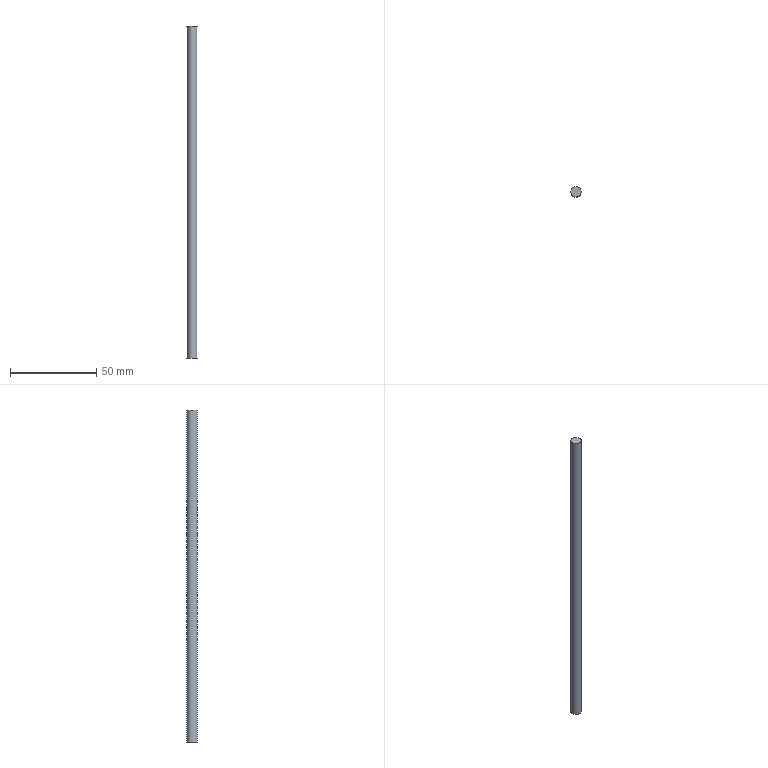Part | NX | features solid 2 | 1 solid | 3 faces | box 6 x 6 x 192 mm | volume 5429 mm3 | plane 2 | cylinder 1 | commonest cylinder face diameters 6 x1
STEP:
#1=CARTESIAN_POINT('',(276.,-28.,-282.));
#2=VERTEX_POINT('',#1);
#3=CARTESIAN_POINT('',(276.,-31.,-282.));
#4=DIRECTION('',(0.,0.,1.));
#5=DIRECTION('',(0.,1.,0.));
#6=AXIS2_PLACEMENT_3D('',#3,#4,#5);
#7=CIRCLE('',#6,3.);
#8=EDGE_CURVE('',#2,#2,#7,.T.);
#9=ORIENTED_EDGE('',*,*,#8,.T.);
#10=EDGE_LOOP('',(#9));
#11=FACE_BOUND('',#10,.T.);
#12=CARTESIAN_POINT('',(276.,-28.,-90.));
#13=VERTEX_POINT('',#12);
#14=CARTESIAN_POINT('',(276.,-31.,-90.));
#15=DIRECTION('',(0.,0.,1.));
#16=DIRECTION('',(0.,1.,0.));
#17=AXIS2_PLACEMENT_3D('',#14,#15,#16);
#18=CIRCLE('',#17,3.);
#19=EDGE_CURVE('',#13,#13,#18,.T.);
#20=ORIENTED_EDGE('',*,*,#19,.F.);
#21=EDGE_LOOP('',(#20));
#22=FACE_BOUND('',#21,.T.);
#23=CARTESIAN_POINT('',(276.,-31.,-282.));
#24=DIRECTION('',(0.,0.,1.));
#25=DIRECTION('',(0.,1.,0.));
#26=AXIS2_PLACEMENT_3D('',#23,#24,#25);
#27=CYLINDRICAL_SURFACE('',#26,3.);
#28=ADVANCED_FACE('',(#11,#22),#27,.T.);
#29=ORIENTED_EDGE('',*,*,#8,.F.);
#30=EDGE_LOOP('',(#29));
#31=FACE_BOUND('',#30,.T.);
#32=CARTESIAN_POINT('',(278.,-33.,-282.));
#33=DIRECTION('',(0.,0.,-1.));
#34=DIRECTION('',(0.,-1.,0.));
#35=AXIS2_PLACEMENT_3D('',#32,#33,#34);
#36=PLANE('',#35);
#37=ADVANCED_FACE('',(#31),#36,.T.);
#38=ORIENTED_EDGE('',*,*,#19,.T.);
#39=EDGE_LOOP('',(#38));
#40=FACE_BOUND('',#39,.T.);
#41=CARTESIAN_POINT('',(278.,-33.,-90.));
#42=DIRECTION('',(0.,0.,-1.));
#43=DIRECTION('',(0.,-1.,0.));
#44=AXIS2_PLACEMENT_3D('',#41,#42,#43);
#45=PLANE('',#44);
#46=ADVANCED_FACE('',(#40),#45,.F.);
#47=CLOSED_SHELL('',(#28,#37,#46));
#48=MANIFOLD_SOLID_BREP('',#47);
#49=(LENGTH_UNIT()NAMED_UNIT(*)SI_UNIT(.MILLI.,.METRE.));
#50=UNCERTAINTY_MEASURE_WITH_UNIT(LENGTH_MEASURE(0.00001),#49,'','');
#51=(NAMED_UNIT(*)PLANE_ANGLE_UNIT()SI_UNIT($,.RADIAN.));
#52=(NAMED_UNIT(*)SI_UNIT($,.STERADIAN.)SOLID_ANGLE_UNIT());
#53=(GEOMETRIC_REPRESENTATION_CONTEXT(3)GLOBAL_UNCERTAINTY_ASSIGNED_CONTEXT((#50))GLOBAL_UNIT_ASSIGNED_CONTEXT((#49,#51,#52))REPRESENTATION_CONTEXT('',''));
#54=ADVANCED_BREP_SHAPE_REPRESENTATION('',(#48),#53);